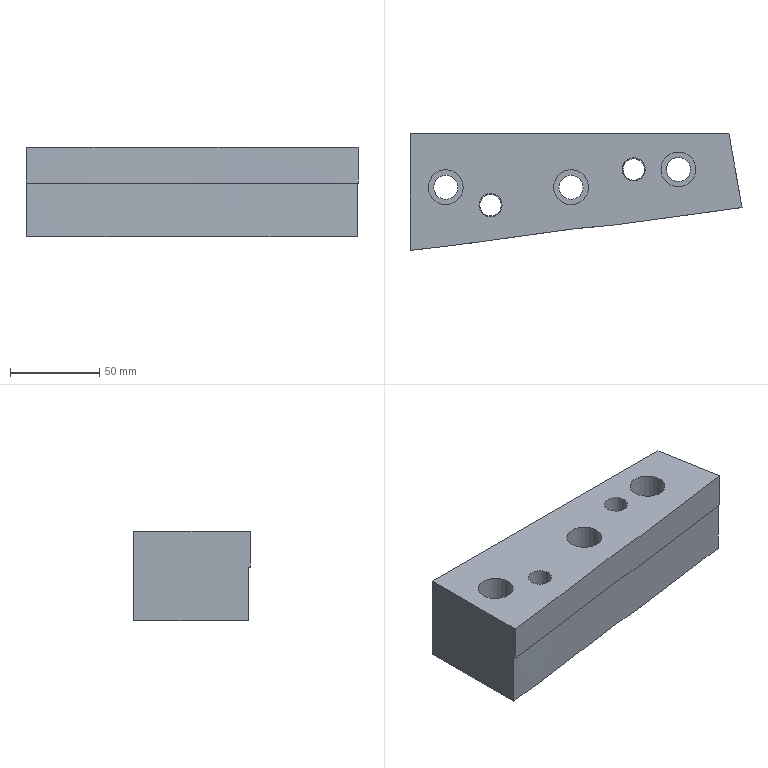Part | NX | features solid 2 | 1 solid | 23 faces | box 185.528 x 65.269 x 50 mm | volume 442182 mm3 | plane 11 | cylinder 10 | spline 2 | commonest cylinder face diameters 13.5 x3 19.5 x3 12 x2 13 x2
STEP:
#1=CARTESIAN_POINT('',(146.,-60.,-50.));
#2=VERTEX_POINT('',#1);
#3=CARTESIAN_POINT('',(140.,-60.,-50.));
#4=DIRECTION('',(0.,0.,1.));
#5=DIRECTION('',(1.,0.,0.));
#6=AXIS2_PLACEMENT_3D('',#3,#4,#5);
#7=CIRCLE('',#6,6.);
#8=EDGE_CURVE('',#2,#2,#7,.T.);
#9=ORIENTED_EDGE('',*,*,#8,.T.);
#10=EDGE_LOOP('',(#9));
#11=FACE_BOUND('',#10,.T.);
#12=CARTESIAN_POINT('',(226.,-40.,-50.));
#13=VERTEX_POINT('',#12);
#14=CARTESIAN_POINT('',(220.,-40.,-50.));
#15=DIRECTION('',(0.,0.,1.));
#16=DIRECTION('',(1.,0.,0.));
#17=AXIS2_PLACEMENT_3D('',#14,#15,#16);
#18=CIRCLE('',#17,6.);
#19=EDGE_CURVE('',#13,#13,#18,.T.);
#20=ORIENTED_EDGE('',*,*,#19,.T.);
#21=EDGE_LOOP('',(#20));
#22=FACE_BOUND('',#21,.T.);
#23=CARTESIAN_POINT('',(121.75,-50.,-50.));
#24=VERTEX_POINT('',#23);
#25=CARTESIAN_POINT('',(115.,-50.,-50.));
#26=DIRECTION('',(0.,0.,1.));
#27=DIRECTION('',(1.,0.,0.));
#28=AXIS2_PLACEMENT_3D('',#25,#26,#27);
#29=CIRCLE('',#28,6.75);
#30=EDGE_CURVE('',#24,#24,#29,.T.);
#31=ORIENTED_EDGE('',*,*,#30,.T.);
#32=EDGE_LOOP('',(#31));
#33=FACE_BOUND('',#32,.T.);
#34=CARTESIAN_POINT('',(191.75,-50.,-50.));
#35=VERTEX_POINT('',#34);
#36=CARTESIAN_POINT('',(185.,-50.,-50.));
#37=DIRECTION('',(0.,0.,1.));
#38=DIRECTION('',(1.,0.,0.));
#39=AXIS2_PLACEMENT_3D('',#36,#37,#38);
#40=CIRCLE('',#39,6.75);
#41=EDGE_CURVE('',#35,#35,#40,.T.);
#42=ORIENTED_EDGE('',*,*,#41,.T.);
#43=EDGE_LOOP('',(#42));
#44=FACE_BOUND('',#43,.T.);
#45=CARTESIAN_POINT('',(251.75,-40.,-50.));
#46=VERTEX_POINT('',#45);
#47=CARTESIAN_POINT('',(245.,-40.,-50.));
#48=DIRECTION('',(0.,0.,1.));
#49=DIRECTION('',(1.,0.,0.));
#50=AXIS2_PLACEMENT_3D('',#47,#48,#49);
#51=CIRCLE('',#50,6.75);
#52=EDGE_CURVE('',#46,#46,#51,.T.);
#53=ORIENTED_EDGE('',*,*,#52,.T.);
#54=EDGE_LOOP('',(#53));
#55=FACE_BOUND('',#54,.T.);
#56=CARTESIAN_POINT('',(280.354,-60.363,-50.));
#57=VERTEX_POINT('',#56);
#58=CARTESIAN_POINT('',(273.237,-20.,-50.));
#59=VERTEX_POINT('',#58);
#60=CARTESIAN_POINT('',(243.048,151.206,-50.));
#61=DIRECTION('',(-0.1736,0.9848,0.));
#62=VECTOR('',#61,1000.);
#63=LINE('',#60,#62);
#64=EDGE_CURVE('',#57,#59,#63,.T.);
#65=ORIENTED_EDGE('',*,*,#64,.F.);
#66=CARTESIAN_POINT('',(95.,-84.264,-50.));
#67=VERTEX_POINT('',#66);
#68=CARTESIAN_POINT('',(280.354,-60.363,-50.));
#69=CARTESIAN_POINT('',(272.636,-61.4,-50.));
#70=CARTESIAN_POINT('',(261.069,-63.03,-50.));
#71=CARTESIAN_POINT('',(245.641,-65.159,-50.));
#72=CARTESIAN_POINT('',(234.064,-66.718,-50.));
#73=CARTESIAN_POINT('',(222.493,-68.314,-50.));
#74=CARTESIAN_POINT('',(210.932,-69.992,-50.));
#75=CARTESIAN_POINT('',(199.277,-70.943,-50.));
#76=CARTESIAN_POINT('',(187.635,-71.985,-50.));
#77=CARTESIAN_POINT('',(176.074,-73.662,-50.));
#78=CARTESIAN_POINT('',(164.507,-75.298,-50.));
#79=CARTESIAN_POINT('',(152.929,-76.84,-50.));
#80=CARTESIAN_POINT('',(137.498,-78.952,-50.));
#81=CARTESIAN_POINT('',(118.23,-81.747,-50.));
#82=CARTESIAN_POINT('',(102.746,-83.443,-50.));
#83=CARTESIAN_POINT('',(95.,-84.264,-50.));
#84=B_SPLINE_CURVE_WITH_KNOTS('',3,(#68,#69,#70,#71,#72,#73,#74,#75,#76,#77,#78,#79,#80,#81,#82,#83),.UNSPECIFIED.,.F.,.F.,(4,1,1,1,1,1,1,1,1,1,1,1,1,4),(0.001298,0.02466,0.03634,0.04802,0.0597,0.07138,0.08306,0.09474,0.1064,0.1181,0.1298,0.1415,0.1648,0.1882),.UNSPECIFIED.);
#85=EDGE_CURVE('',#57,#67,#84,.T.);
#86=ORIENTED_EDGE('',*,*,#85,.T.);
#87=CARTESIAN_POINT('',(95.,-20.,-50.));
#88=VERTEX_POINT('',#87);
#89=CARTESIAN_POINT('',(95.,35.09,-50.));
#90=DIRECTION('',(0.,1.,0.));
#91=VECTOR('',#90,1000.);
#92=LINE('',#89,#91);
#93=EDGE_CURVE('',#67,#88,#92,.T.);
#94=ORIENTED_EDGE('',*,*,#93,.T.);
#95=CARTESIAN_POINT('',(-415.478,-20.,-50.));
#96=DIRECTION('',(-1.,0.,0.));
#97=VECTOR('',#96,1000.);
#98=LINE('',#95,#97);
#99=EDGE_CURVE('',#59,#88,#98,.T.);
#100=ORIENTED_EDGE('',*,*,#99,.F.);
#101=EDGE_LOOP('',(#65,#86,#94,#100));
#102=FACE_BOUND('',#101,.T.);
#103=CARTESIAN_POINT('',(-415.478,35.09,-50.));
#104=DIRECTION('',(0.,0.,1.));
#105=DIRECTION('',(1.,0.,0.));
#106=AXIS2_PLACEMENT_3D('',#103,#104,#105);
#107=PLANE('',#106);
#108=ADVANCED_FACE('',(#11,#22,#33,#44,#55,#102),#107,.F.);
#109=CARTESIAN_POINT('',(280.354,-60.363,-20.));
#110=VERTEX_POINT('',#109);
#111=CARTESIAN_POINT('',(280.528,-61.349,-20.));
#112=VERTEX_POINT('',#111);
#113=CARTESIAN_POINT('',(298.119,-161.113,-20.));
#114=DIRECTION('',(0.1736,-0.9848,0.));
#115=VECTOR('',#114,1000.);
#116=LINE('',#113,#115);
#117=EDGE_CURVE('',#110,#112,#116,.T.);
#118=ORIENTED_EDGE('',*,*,#117,.F.);
#119=CARTESIAN_POINT('',(280.354,-60.363,-60.));
#120=DIRECTION('',(0.,0.,-1.));
#121=VECTOR('',#120,1000.);
#122=LINE('',#119,#121);
#123=EDGE_CURVE('',#57,#110,#122,.F.);
#124=ORIENTED_EDGE('',*,*,#123,.F.);
#125=ORIENTED_EDGE('',*,*,#64,.T.);
#126=CARTESIAN_POINT('',(273.237,-20.,0.));
#127=VERTEX_POINT('',#126);
#128=CARTESIAN_POINT('',(273.237,-20.,0.));
#129=DIRECTION('',(0.,0.,-1.));
#130=VECTOR('',#129,1000.);
#131=LINE('',#128,#130);
#132=EDGE_CURVE('',#127,#59,#131,.T.);
#133=ORIENTED_EDGE('',*,*,#132,.F.);
#134=CARTESIAN_POINT('',(280.528,-61.349,0.));
#135=VERTEX_POINT('',#134);
#136=CARTESIAN_POINT('',(285.358,-88.743,0.));
#137=DIRECTION('',(0.1736,-0.9848,0.));
#138=VECTOR('',#137,1000.);
#139=LINE('',#136,#138);
#140=EDGE_CURVE('',#127,#135,#139,.T.);
#141=ORIENTED_EDGE('',*,*,#140,.T.);
#142=CARTESIAN_POINT('',(280.528,-61.349,-10.));
#143=DIRECTION('',(0.,0.,-1.));
#144=VECTOR('',#143,1000.);
#145=LINE('',#142,#144);
#146=EDGE_CURVE('',#135,#112,#145,.T.);
#147=ORIENTED_EDGE('',*,*,#146,.T.);
#148=EDGE_LOOP('',(#118,#124,#125,#133,#141,#147));
#149=FACE_BOUND('',#148,.T.);
#150=CARTESIAN_POINT('',(298.119,-161.113,0.));
#151=DIRECTION('',(0.9848,0.1736,0.));
#152=DIRECTION('',(-0.1736,0.9848,0.));
#153=AXIS2_PLACEMENT_3D('',#150,#151,#152);
#154=PLANE('',#153);
#155=ADVANCED_FACE('',(#149),#154,.T.);
#156=CARTESIAN_POINT('',(95.,-20.,0.));
#157=VERTEX_POINT('',#156);
#158=CARTESIAN_POINT('',(-470.381,-20.,0.));
#159=DIRECTION('',(1.,0.,0.));
#160=VECTOR('',#159,1000.);
#161=LINE('',#158,#160);
#162=EDGE_CURVE('',#157,#127,#161,.T.);
#163=ORIENTED_EDGE('',*,*,#162,.T.);
#164=ORIENTED_EDGE('',*,*,#132,.T.);
#165=ORIENTED_EDGE('',*,*,#99,.T.);
#166=CARTESIAN_POINT('',(95.,-20.,0.));
#167=DIRECTION('',(0.,0.,-1.));
#168=VECTOR('',#167,1000.);
#169=LINE('',#166,#168);
#170=EDGE_CURVE('',#157,#88,#169,.T.);
#171=ORIENTED_EDGE('',*,*,#170,.F.);
#172=EDGE_LOOP('',(#163,#164,#165,#171));
#173=FACE_BOUND('',#172,.T.);
#174=CARTESIAN_POINT('',(190.,-20.,0.));
#175=DIRECTION('',(0.,1.,0.));
#176=DIRECTION('',(0.,0.,1.));
#177=AXIS2_PLACEMENT_3D('',#174,#175,#176);
#178=PLANE('',#177);
#179=ADVANCED_FACE('',(#173),#178,.T.);
#180=CARTESIAN_POINT('',(95.,-85.269,0.));
#181=VERTEX_POINT('',#180);
#182=CARTESIAN_POINT('',(95.,-85.269,-20.));
#183=VERTEX_POINT('',#182);
#184=CARTESIAN_POINT('',(95.,-85.269,-10.));
#185=DIRECTION('',(0.,0.,-1.));
#186=VECTOR('',#185,1000.);
#187=LINE('',#184,#186);
#188=EDGE_CURVE('',#181,#183,#187,.T.);
#189=ORIENTED_EDGE('',*,*,#188,.T.);
#190=CARTESIAN_POINT('',(-190.231,-121.49,-20.));
#191=CARTESIAN_POINT('',(-188.654,-121.152,-20.));
#192=CARTESIAN_POINT('',(-185.47,-120.627,-20.));
#193=CARTESIAN_POINT('',(-180.656,-120.141,-20.));
#194=CARTESIAN_POINT('',(-175.882,-119.326,-20.));
#195=CARTESIAN_POINT('',(-169.679,-117.528,-20.));
#196=CARTESIAN_POINT('',(-162.185,-114.539,-20.));
#197=CARTESIAN_POINT('',(-153.086,-111.254,-20.));
#198=CARTESIAN_POINT('',(-144.031,-107.845,-20.));
#199=CARTESIAN_POINT('',(-136.465,-105.061,-20.));
#200=CARTESIAN_POINT('',(-130.418,-102.814,-20.));
#201=CARTESIAN_POINT('',(-125.812,-101.329,-20.));
#202=CARTESIAN_POINT('',(-121.306,-99.566,-20.));
#203=CARTESIAN_POINT('',(-116.876,-97.626,-20.));
#204=CARTESIAN_POINT('',(-112.335,-95.923,-20.));
#205=CARTESIAN_POINT('',(-107.564,-95.05,-20.));
#206=CARTESIAN_POINT('',(-102.756,-94.525,-20.));
#207=CARTESIAN_POINT('',(-96.349,-93.771,-20.));
#208=CARTESIAN_POINT('',(-89.902,-93.468,-20.));
#209=CARTESIAN_POINT('',(-83.452,-93.448,-20.));
#210=CARTESIAN_POINT('',(-77.002,-93.469,-20.));
#211=CARTESIAN_POINT('',(-68.939,-93.411,-20.));
#212=CARTESIAN_POINT('',(-56.04,-93.3,-20.));
#213=CARTESIAN_POINT('',(-33.465,-93.184,-20.));
#214=CARTESIAN_POINT('',(-7.666,-93.074,-20.));
#215=CARTESIAN_POINT('',(14.907,-92.653,-20.));
#216=CARTESIAN_POINT('',(27.794,-92.068,-20.));
#217=CARTESIAN_POINT('',(40.668,-91.245,-20.));
#218=CARTESIAN_POINT('',(51.917,-90.291,-20.));
#219=CARTESIAN_POINT('',(61.528,-89.174,-20.));
#220=CARTESIAN_POINT('',(67.939,-88.466,-20.));
#221=CARTESIAN_POINT('',(79.125,-86.95,-20.));
#222=CARTESIAN_POINT('',(95.161,-85.253,-20.));
#223=CARTESIAN_POINT('',(114.404,-83.21,-20.));
#224=CARTESIAN_POINT('',(133.568,-80.524,-20.));
#225=CARTESIAN_POINT('',(152.734,-77.861,-20.));
#226=CARTESIAN_POINT('',(171.916,-75.326,-20.));
#227=CARTESIAN_POINT('',(191.055,-72.413,-20.));
#228=CARTESIAN_POINT('',(207.17,-71.468,-20.));
#229=CARTESIAN_POINT('',(219.951,-69.697,-20.));
#230=CARTESIAN_POINT('',(232.724,-67.899,-20.));
#231=CARTESIAN_POINT('',(248.708,-65.766,-20.));
#232=CARTESIAN_POINT('',(267.87,-63.074,-20.));
#233=CARTESIAN_POINT('',(287.038,-60.44,-20.));
#234=CARTESIAN_POINT('',(301.448,-58.682,-20.));
#235=CARTESIAN_POINT('',(310.976,-56.987,-20.));
#236=CARTESIAN_POINT('',(314.916,-56.135,-20.));
#237=CARTESIAN_POINT('',(318.052,-55.382,-20.));
#238=CARTESIAN_POINT('',(320.39,-54.76,-20.));
#239=CARTESIAN_POINT('',(322.686,-53.981,-20.));
#240=CARTESIAN_POINT('',(325.595,-52.578,-20.));
#241=CARTESIAN_POINT('',(328.769,-50.098,-20.));
#242=CARTESIAN_POINT('',(332.247,-46.69,-20.));
#243=CARTESIAN_POINT('',(335.795,-43.406,-20.));
#244=CARTESIAN_POINT('',(343.661,-37.758,-20.));
#245=CARTESIAN_POINT('',(355.164,-28.914,-20.));
#246=CARTESIAN_POINT('',(370.422,-17.018,-20.));
#247=CARTESIAN_POINT('',(383.264,-7.249,-20.));
#248=CARTESIAN_POINT('',(392.416,-0.6713,-20.));
#249=CARTESIAN_POINT('',(396.953,2.733,-20.));
#250=CARTESIAN_POINT('',(398.886,5.372,-20.));
#251=CARTESIAN_POINT('',(399.725,7.654,-20.));
#252=CARTESIAN_POINT('',(399.76,10.078,-20.));
#253=CARTESIAN_POINT('',(399.483,13.317,-20.));
#254=CARTESIAN_POINT('',(399.712,17.34,-20.));
#255=CARTESIAN_POINT('',(399.612,22.179,-20.));
#256=CARTESIAN_POINT('',(399.633,31.854,-20.));
#257=CARTESIAN_POINT('',(399.593,46.366,-20.));
#258=CARTESIAN_POINT('',(399.637,62.491,-20.));
#259=CARTESIAN_POINT('',(399.588,73.779,-20.));
#260=CARTESIAN_POINT('',(399.652,79.422,-20.));
#261=CARTESIAN_POINT('',(399.59,82.647,-20.));
#262=CARTESIAN_POINT('',(399.564,85.065,-20.));
#263=CARTESIAN_POINT('',(399.725,87.486,-20.));
#264=CARTESIAN_POINT('',(399.756,89.902,-20.));
#265=CARTESIAN_POINT('',(399.247,92.301,-20.));
#266=CARTESIAN_POINT('',(397.362,95.008,-20.));
#267=CARTESIAN_POINT('',(393.635,96.774,-20.));
#268=CARTESIAN_POINT('',(389.279,98.826,-20.));
#269=CARTESIAN_POINT('',(384.732,100.498,-20.));
#270=CARTESIAN_POINT('',(378.765,102.95,-20.));
#271=CARTESIAN_POINT('',(362.589,110.229,-20.));
#272=CARTESIAN_POINT('',(344.928,118.135,-20.));
#273=CARTESIAN_POINT('',(327.281,126.072,-20.));
#274=CARTESIAN_POINT('',(319.932,129.381,-20.));
#275=CARTESIAN_POINT('',(314.075,132.102,-20.));
#276=CARTESIAN_POINT('',(309.387,133.376,-20.));
#277=CARTESIAN_POINT('',(304.547,133.785,-20.));
#278=CARTESIAN_POINT('',(299.716,133.401,-20.));
#279=CARTESIAN_POINT('',(294.929,132.704,-20.));
#280=CARTESIAN_POINT('',(288.543,131.8,-20.));
#281=CARTESIAN_POINT('',(277.364,130.241,-20.));
#282=CARTESIAN_POINT('',(242.2,125.552,-20.));
#283=CARTESIAN_POINT('',(184.637,118.048,-20.));
#284=CARTESIAN_POINT('',(120.701,109.541,-20.));
#285=CARTESIAN_POINT('',(69.531,102.902,-20.));
#286=CARTESIAN_POINT('',(40.777,98.94,-20.));
#287=CARTESIAN_POINT('',(21.566,96.615,-20.));
#288=CARTESIAN_POINT('',(8.743,95.212,-20.));
#289=CARTESIAN_POINT('',(-7.301,93.575,-20.));
#290=CARTESIAN_POINT('',(-26.625,92.505,-20.));
#291=CARTESIAN_POINT('',(-45.971,92.017,-20.));
#292=CARTESIAN_POINT('',(-62.09,91.675,-20.));
#293=CARTESIAN_POINT('',(-74.987,91.256,-20.));
#294=CARTESIAN_POINT('',(-84.664,91.165,-20.));
#295=CARTESIAN_POINT('',(-94.319,91.781,-20.));
#296=CARTESIAN_POINT('',(-103.929,92.966,-20.));
#297=CARTESIAN_POINT('',(-113.495,94.403,-20.));
#298=CARTESIAN_POINT('',(-119.856,95.492,-20.));
#299=CARTESIAN_POINT('',(-122.997,96.222,-20.));
#300=B_SPLINE_CURVE_WITH_KNOTS('',3,(#190,#191,#192,#193,#194,#195,#196,#197,#198,#199,#200,#201,#202,#203,#204,#205,#206,#207,#208,#209,#210,#211,#212,#213,#214,#215,#216,#217,#218,#219,#220,#221,#222,#223,#224,#225,#226,#227,#228,#229,#230,#231,#232,#233,#234,#235,#236,#237,#238,#239,#240,#241,#242,#243,#244,#245,#246,#247,#248,#249,#250,#251,#252,#253,#254,#255,#256,#257,#258,#259,#260,#261,#262,#263,#264,#265,#266,#267,#268,#269,#270,#271,#272,#273,#274,#275,#276,#277,#278,#279,#280,#281,#282,#283,#284,#285,#286,#287,#288,#289,#290,#291,#292,#293,#294,#295,#296,#297,#298,#299),.UNSPECIFIED.,.F.,.F.,(4,1,1,1,1,1,1,1,1,1,1,1,1,1,1,1,1,1,1,1,1,1,1,1,1,1,1,1,1,1,1,1,1,1,1,1,1,1,1,1,1,1,1,1,1,1,1,1,1,1,1,1,1,1,1,1,1,1,1,1,1,1,1,1,1,1,1,1,1,1,1,1,1,1,1,1,1,1,1,1,1,1,1,1,1,1,1,1,1,1,1,1,1,1,1,1,1,1,1,1,1,1,1,1,1,1,1,4),(0.4704,0.4724,0.4745,0.4766,0.4786,0.4828,0.4869,0.491,0.4952,0.4972,0.4993,0.5014,0.5035,0.5055,0.5076,0.5097,0.5117,0.5159,0.5179,0.52,0.5241,0.5283,0.5366,0.5531,0.5614,0.5655,0.5697,0.5779,0.58,0.5821,0.5862,0.5945,0.6028,0.611,0.6193,0.6276,0.6359,0.6441,0.6483,0.6524,0.6607,0.669,0.6772,0.6855,0.6876,0.6897,0.6907,0.6917,0.6928,0.6938,0.6959,0.6979,0.7,0.7021,0.7103,0.7186,0.7269,0.731,0.7331,0.7341,0.7352,0.7362,0.7372,0.7393,0.7414,0.7435,0.7517,0.76,0.7641,0.7662,0.7672,0.7683,0.7693,0.7703,0.7714,0.7724,0.7745,0.7766,0.7786,0.7807,0.7848,0.8014,0.8055,0.8097,0.8117,0.8138,0.8159,0.8179,0.82,0.8221,0.8262,0.8345,0.8676,0.9007,0.9172,0.9338,0.9379,0.9421,0.9503,0.9586,0.9669,0.9752,0.9793,0.9834,0.9876,0.9917,0.9959,1.),.UNSPECIFIED.);
#301=EDGE_CURVE('',#183,#112,#300,.T.);
#302=ORIENTED_EDGE('',*,*,#301,.T.);
#303=ORIENTED_EDGE('',*,*,#146,.F.);
#304=CARTESIAN_POINT('',(280.528,-61.349,0.));
#305=CARTESIAN_POINT('',(272.803,-62.386,0.));
#306=CARTESIAN_POINT('',(261.225,-64.018,0.));
#307=CARTESIAN_POINT('',(245.782,-66.149,0.));
#308=CARTESIAN_POINT('',(234.195,-67.709,0.));
#309=CARTESIAN_POINT('',(222.613,-69.308,0.));
#310=CARTESIAN_POINT('',(211.041,-70.986,0.));
#311=CARTESIAN_POINT('',(199.375,-71.938,0.));
#312=CARTESIAN_POINT('',(187.722,-72.982,0.));
#313=CARTESIAN_POINT('',(176.15,-74.662,0.));
#314=CARTESIAN_POINT('',(164.573,-76.298,0.));
#315=CARTESIAN_POINT('',(152.984,-77.842,0.));
#316=CARTESIAN_POINT('',(137.539,-79.956,0.));
#317=CARTESIAN_POINT('',(118.252,-82.754,0.));
#318=CARTESIAN_POINT('',(102.753,-84.448,0.));
#319=CARTESIAN_POINT('',(95.,-85.269,0.));
#320=B_SPLINE_CURVE_WITH_KNOTS('',3,(#304,#305,#306,#307,#308,#309,#310,#311,#312,#313,#314,#315,#316,#317,#318,#319),.UNSPECIFIED.,.F.,.F.,(4,1,1,1,1,1,1,1,1,1,1,1,1,4),(0.,0.02338,0.03507,0.04677,0.05846,0.07015,0.08184,0.09353,0.1052,0.1169,0.1286,0.1403,0.1637,0.1871),.UNSPECIFIED.);
#321=EDGE_CURVE('',#135,#181,#320,.T.);
#322=ORIENTED_EDGE('',*,*,#321,.T.);
#323=EDGE_LOOP('',(#189,#302,#303,#322));
#324=FACE_BOUND('',#323,.T.);
#325=CARTESIAN_POINT('',(95.,-85.269,0.));
#326=CARTESIAN_POINT('',(95.,-85.269,-20.));
#327=CARTESIAN_POINT('',(102.752,-84.448,0.));
#328=CARTESIAN_POINT('',(102.752,-84.448,-20.));
#329=CARTESIAN_POINT('',(118.251,-82.754,0.));
#330=CARTESIAN_POINT('',(118.251,-82.754,-20.));
#331=CARTESIAN_POINT('',(137.54,-79.956,0.));
#332=CARTESIAN_POINT('',(137.54,-79.956,-20.));
#333=CARTESIAN_POINT('',(152.986,-77.841,0.));
#334=CARTESIAN_POINT('',(152.986,-77.841,-20.));
#335=CARTESIAN_POINT('',(164.576,-76.298,0.));
#336=CARTESIAN_POINT('',(164.576,-76.298,-20.));
#337=CARTESIAN_POINT('',(176.156,-74.661,0.));
#338=CARTESIAN_POINT('',(176.156,-74.661,-20.));
#339=CARTESIAN_POINT('',(187.73,-72.981,0.));
#340=CARTESIAN_POINT('',(187.73,-72.981,-20.));
#341=CARTESIAN_POINT('',(199.376,-71.938,0.));
#342=CARTESIAN_POINT('',(199.376,-71.938,-20.));
#343=CARTESIAN_POINT('',(211.033,-70.987,0.));
#344=CARTESIAN_POINT('',(211.033,-70.987,-20.));
#345=CARTESIAN_POINT('',(222.609,-69.308,0.));
#346=CARTESIAN_POINT('',(222.609,-69.308,-20.));
#347=CARTESIAN_POINT('',(234.191,-67.71,0.));
#348=CARTESIAN_POINT('',(234.191,-67.71,-20.));
#349=CARTESIAN_POINT('',(245.779,-66.15,0.));
#350=CARTESIAN_POINT('',(245.779,-66.15,-20.));
#351=CARTESIAN_POINT('',(261.224,-64.018,0.));
#352=CARTESIAN_POINT('',(261.224,-64.018,-20.));
#353=CARTESIAN_POINT('',(272.802,-62.386,0.));
#354=CARTESIAN_POINT('',(272.802,-62.386,-20.));
#355=CARTESIAN_POINT('',(280.528,-61.349,0.));
#356=CARTESIAN_POINT('',(280.528,-61.349,-20.));
#357=B_SPLINE_SURFACE_WITH_KNOTS('',3,1,((#325,#326),(#327,#328),(#329,#330),(#331,#332),(#333,#334),(#335,#336),(#337,#338),(#339,#340),(#341,#342),(#343,#344),(#345,#346),(#347,#348),(#349,#350),(#351,#352),(#353,#354),(#355,#356)),.SURF_OF_LINEAR_EXTRUSION.,.F.,.F.,.F.,(4,1,1,1,1,1,1,1,1,1,1,1,1,4),(2,2),(0.5944,0.6044,0.6144,0.6194,0.6244,0.6294,0.6344,0.6394,0.6444,0.6494,0.6544,0.6594,0.6644,0.6744),(0.,1.),.UNSPECIFIED.);
#358=ADVANCED_FACE('',(#324),#357,.F.);
#359=CARTESIAN_POINT('',(133.5,-60.,0.));
#360=VERTEX_POINT('',#359);
#361=CARTESIAN_POINT('',(140.,-60.,0.));
#362=DIRECTION('',(0.,0.,-1.));
#363=DIRECTION('',(-1.,0.,0.));
#364=AXIS2_PLACEMENT_3D('',#361,#362,#363);
#365=CIRCLE('',#364,6.5);
#366=EDGE_CURVE('',#360,#360,#365,.T.);
#367=ORIENTED_EDGE('',*,*,#366,.T.);
#368=EDGE_LOOP('',(#367));
#369=FACE_BOUND('',#368,.T.);
#370=CARTESIAN_POINT('',(213.5,-40.,0.));
#371=VERTEX_POINT('',#370);
#372=CARTESIAN_POINT('',(220.,-40.,0.));
#373=DIRECTION('',(0.,0.,-1.));
#374=DIRECTION('',(-1.,0.,0.));
#375=AXIS2_PLACEMENT_3D('',#372,#373,#374);
#376=CIRCLE('',#375,6.5);
#377=EDGE_CURVE('',#371,#371,#376,.T.);
#378=ORIENTED_EDGE('',*,*,#377,.T.);
#379=EDGE_LOOP('',(#378));
#380=FACE_BOUND('',#379,.T.);
#381=CARTESIAN_POINT('',(105.25,-50.,0.));
#382=VERTEX_POINT('',#381);
#383=CARTESIAN_POINT('',(115.,-50.,0.));
#384=DIRECTION('',(0.,0.,-1.));
#385=DIRECTION('',(-1.,0.,0.));
#386=AXIS2_PLACEMENT_3D('',#383,#384,#385);
#387=CIRCLE('',#386,9.75);
#388=EDGE_CURVE('',#382,#382,#387,.T.);
#389=ORIENTED_EDGE('',*,*,#388,.T.);
#390=EDGE_LOOP('',(#389));
#391=FACE_BOUND('',#390,.T.);
#392=CARTESIAN_POINT('',(175.25,-50.,0.));
#393=VERTEX_POINT('',#392);
#394=CARTESIAN_POINT('',(185.,-50.,0.));
#395=DIRECTION('',(0.,0.,-1.));
#396=DIRECTION('',(-1.,0.,0.));
#397=AXIS2_PLACEMENT_3D('',#394,#395,#396);
#398=CIRCLE('',#397,9.75);
#399=EDGE_CURVE('',#393,#393,#398,.T.);
#400=ORIENTED_EDGE('',*,*,#399,.T.);
#401=EDGE_LOOP('',(#400));
#402=FACE_BOUND('',#401,.T.);
#403=CARTESIAN_POINT('',(235.25,-40.,0.));
#404=VERTEX_POINT('',#403);
#405=CARTESIAN_POINT('',(245.,-40.,0.));
#406=DIRECTION('',(0.,0.,-1.));
#407=DIRECTION('',(-1.,0.,0.));
#408=AXIS2_PLACEMENT_3D('',#405,#406,#407);
#409=CIRCLE('',#408,9.75);
#410=EDGE_CURVE('',#404,#404,#409,.T.);
#411=ORIENTED_EDGE('',*,*,#410,.T.);
#412=EDGE_LOOP('',(#411));
#413=FACE_BOUND('',#412,.T.);
#414=ORIENTED_EDGE('',*,*,#140,.F.);
#415=ORIENTED_EDGE('',*,*,#162,.F.);
#416=CARTESIAN_POINT('',(95.,-222.,0.));
#417=DIRECTION('',(0.,-1.,0.));
#418=VECTOR('',#417,1000.);
#419=LINE('',#416,#418);
#420=EDGE_CURVE('',#157,#181,#419,.T.);
#421=ORIENTED_EDGE('',*,*,#420,.T.);
#422=ORIENTED_EDGE('',*,*,#321,.F.);
#423=EDGE_LOOP('',(#414,#415,#421,#422));
#424=FACE_BOUND('',#423,.T.);
#425=CARTESIAN_POINT('',(-470.381,-222.,0.));
#426=DIRECTION('',(0.,0.,-1.));
#427=DIRECTION('',(-1.,0.,0.));
#428=AXIS2_PLACEMENT_3D('',#425,#426,#427);
#429=PLANE('',#428);
#430=ADVANCED_FACE('',(#369,#380,#391,#402,#413,#424),#429,.F.);
#431=CARTESIAN_POINT('',(95.,-84.264,-20.));
#432=VERTEX_POINT('',#431);
#433=CARTESIAN_POINT('',(95.,-84.264,-60.));
#434=DIRECTION('',(0.,0.,-1.));
#435=VECTOR('',#434,1000.);
#436=LINE('',#433,#435);
#437=EDGE_CURVE('',#67,#432,#436,.F.);
#438=ORIENTED_EDGE('',*,*,#437,.T.);
#439=CARTESIAN_POINT('',(95.,83.097,-20.));
#440=DIRECTION('',(0.,-1.,0.));
#441=VECTOR('',#440,1000.);
#442=LINE('',#439,#441);
#443=EDGE_CURVE('',#432,#183,#442,.T.);
#444=ORIENTED_EDGE('',*,*,#443,.T.);
#445=ORIENTED_EDGE('',*,*,#188,.F.);
#446=ORIENTED_EDGE('',*,*,#420,.F.);
#447=ORIENTED_EDGE('',*,*,#170,.T.);
#448=ORIENTED_EDGE('',*,*,#93,.F.);
#449=EDGE_LOOP('',(#438,#444,#445,#446,#447,#448));
#450=FACE_BOUND('',#449,.T.);
#451=CARTESIAN_POINT('',(95.,83.097,-25.));
#452=DIRECTION('',(1.,0.,0.));
#453=DIRECTION('',(0.,0.,-1.));
#454=AXIS2_PLACEMENT_3D('',#451,#452,#453);
#455=PLANE('',#454);
#456=ADVANCED_FACE('',(#450),#455,.F.);
#457=CARTESIAN_POINT('',(238.25,-40.,-15.));
#458=VERTEX_POINT('',#457);
#459=CARTESIAN_POINT('',(245.,-40.,-15.));
#460=DIRECTION('',(0.,0.,-1.));
#461=DIRECTION('',(-1.,0.,0.));
#462=AXIS2_PLACEMENT_3D('',#459,#460,#461);
#463=CIRCLE('',#462,6.75);
#464=EDGE_CURVE('',#458,#458,#463,.T.);
#465=ORIENTED_EDGE('',*,*,#464,.F.);
#466=EDGE_LOOP('',(#465));
#467=FACE_BOUND('',#466,.T.);
#468=ORIENTED_EDGE('',*,*,#52,.F.);
#469=EDGE_LOOP('',(#468));
#470=FACE_BOUND('',#469,.T.);
#471=CARTESIAN_POINT('',(245.,-40.,-100.));
#472=DIRECTION('',(0.,0.,-1.));
#473=DIRECTION('',(-1.,0.,0.));
#474=AXIS2_PLACEMENT_3D('',#471,#472,#473);
#475=CYLINDRICAL_SURFACE('',#474,6.75);
#476=ADVANCED_FACE('',(#467,#470),#475,.F.);
#477=ORIENTED_EDGE('',*,*,#464,.T.);
#478=EDGE_LOOP('',(#477));
#479=FACE_BOUND('',#478,.T.);
#480=CARTESIAN_POINT('',(235.25,-40.,-15.));
#481=VERTEX_POINT('',#480);
#482=CARTESIAN_POINT('',(245.,-40.,-15.));
#483=DIRECTION('',(0.,0.,-1.));
#484=DIRECTION('',(-1.,0.,0.));
#485=AXIS2_PLACEMENT_3D('',#482,#483,#484);
#486=CIRCLE('',#485,9.75);
#487=EDGE_CURVE('',#481,#481,#486,.T.);
#488=ORIENTED_EDGE('',*,*,#487,.F.);
#489=EDGE_LOOP('',(#488));
#490=FACE_BOUND('',#489,.T.);
#491=CARTESIAN_POINT('',(245.,-40.,-15.));
#492=DIRECTION('',(0.,0.,-1.));
#493=DIRECTION('',(-1.,0.,0.));
#494=AXIS2_PLACEMENT_3D('',#491,#492,#493);
#495=PLANE('',#494);
#496=ADVANCED_FACE('',(#479,#490),#495,.F.);
#497=ORIENTED_EDGE('',*,*,#487,.T.);
#498=EDGE_LOOP('',(#497));
#499=FACE_BOUND('',#498,.T.);
#500=ORIENTED_EDGE('',*,*,#410,.F.);
#501=EDGE_LOOP('',(#500));
#502=FACE_BOUND('',#501,.T.);
#503=CARTESIAN_POINT('',(245.,-40.,0.));
#504=DIRECTION('',(0.,0.,-1.));
#505=DIRECTION('',(-1.,0.,0.));
#506=AXIS2_PLACEMENT_3D('',#503,#504,#505);
#507=CYLINDRICAL_SURFACE('',#506,9.75);
#508=ADVANCED_FACE('',(#499,#502),#507,.F.);
#509=CARTESIAN_POINT('',(178.25,-50.,-15.));
#510=VERTEX_POINT('',#509);
#511=CARTESIAN_POINT('',(185.,-50.,-15.));
#512=DIRECTION('',(0.,0.,-1.));
#513=DIRECTION('',(-1.,0.,0.));
#514=AXIS2_PLACEMENT_3D('',#511,#512,#513);
#515=CIRCLE('',#514,6.75);
#516=EDGE_CURVE('',#510,#510,#515,.T.);
#517=ORIENTED_EDGE('',*,*,#516,.F.);
#518=EDGE_LOOP('',(#517));
#519=FACE_BOUND('',#518,.T.);
#520=ORIENTED_EDGE('',*,*,#41,.F.);
#521=EDGE_LOOP('',(#520));
#522=FACE_BOUND('',#521,.T.);
#523=CARTESIAN_POINT('',(185.,-50.,-100.));
#524=DIRECTION('',(0.,0.,-1.));
#525=DIRECTION('',(-1.,0.,0.));
#526=AXIS2_PLACEMENT_3D('',#523,#524,#525);
#527=CYLINDRICAL_SURFACE('',#526,6.75);
#528=ADVANCED_FACE('',(#519,#522),#527,.F.);
#529=ORIENTED_EDGE('',*,*,#516,.T.);
#530=EDGE_LOOP('',(#529));
#531=FACE_BOUND('',#530,.T.);
#532=CARTESIAN_POINT('',(175.25,-50.,-15.));
#533=VERTEX_POINT('',#532);
#534=CARTESIAN_POINT('',(185.,-50.,-15.));
#535=DIRECTION('',(0.,0.,-1.));
#536=DIRECTION('',(-1.,0.,0.));
#537=AXIS2_PLACEMENT_3D('',#534,#535,#536);
#538=CIRCLE('',#537,9.75);
#539=EDGE_CURVE('',#533,#533,#538,.T.);
#540=ORIENTED_EDGE('',*,*,#539,.F.);
#541=EDGE_LOOP('',(#540));
#542=FACE_BOUND('',#541,.T.);
#543=CARTESIAN_POINT('',(185.,-60.,-15.));
#544=DIRECTION('',(0.,0.,-1.));
#545=DIRECTION('',(-1.,0.,0.));
#546=AXIS2_PLACEMENT_3D('',#543,#544,#545);
#547=PLANE('',#546);
#548=ADVANCED_FACE('',(#531,#542),#547,.F.);
#549=ORIENTED_EDGE('',*,*,#539,.T.);
#550=EDGE_LOOP('',(#549));
#551=FACE_BOUND('',#550,.T.);
#552=ORIENTED_EDGE('',*,*,#399,.F.);
#553=EDGE_LOOP('',(#552));
#554=FACE_BOUND('',#553,.T.);
#555=CARTESIAN_POINT('',(185.,-50.,0.));
#556=DIRECTION('',(0.,0.,-1.));
#557=DIRECTION('',(-1.,0.,0.));
#558=AXIS2_PLACEMENT_3D('',#555,#556,#557);
#559=CYLINDRICAL_SURFACE('',#558,9.75);
#560=ADVANCED_FACE('',(#551,#554),#559,.F.);
#561=CARTESIAN_POINT('',(108.25,-50.,-15.));
#562=VERTEX_POINT('',#561);
#563=CARTESIAN_POINT('',(115.,-50.,-15.));
#564=DIRECTION('',(0.,0.,-1.));
#565=DIRECTION('',(-1.,0.,0.));
#566=AXIS2_PLACEMENT_3D('',#563,#564,#565);
#567=CIRCLE('',#566,6.75);
#568=EDGE_CURVE('',#562,#562,#567,.T.);
#569=ORIENTED_EDGE('',*,*,#568,.F.);
#570=EDGE_LOOP('',(#569));
#571=FACE_BOUND('',#570,.T.);
#572=ORIENTED_EDGE('',*,*,#30,.F.);
#573=EDGE_LOOP('',(#572));
#574=FACE_BOUND('',#573,.T.);
#575=CARTESIAN_POINT('',(115.,-50.,-100.));
#576=DIRECTION('',(0.,0.,-1.));
#577=DIRECTION('',(-1.,0.,0.));
#578=AXIS2_PLACEMENT_3D('',#575,#576,#577);
#579=CYLINDRICAL_SURFACE('',#578,6.75);
#580=ADVANCED_FACE('',(#571,#574),#579,.F.);
#581=ORIENTED_EDGE('',*,*,#568,.T.);
#582=EDGE_LOOP('',(#581));
#583=FACE_BOUND('',#582,.T.);
#584=CARTESIAN_POINT('',(105.25,-50.,-15.));
#585=VERTEX_POINT('',#584);
#586=CARTESIAN_POINT('',(115.,-50.,-15.));
#587=DIRECTION('',(0.,0.,-1.));
#588=DIRECTION('',(-1.,0.,0.));
#589=AXIS2_PLACEMENT_3D('',#586,#587,#588);
#590=CIRCLE('',#589,9.75);
#591=EDGE_CURVE('',#585,#585,#590,.T.);
#592=ORIENTED_EDGE('',*,*,#591,.F.);
#593=EDGE_LOOP('',(#592));
#594=FACE_BOUND('',#593,.T.);
#595=CARTESIAN_POINT('',(115.,-50.,-15.));
#596=DIRECTION('',(0.,0.,-1.));
#597=DIRECTION('',(-1.,0.,0.));
#598=AXIS2_PLACEMENT_3D('',#595,#596,#597);
#599=PLANE('',#598);
#600=ADVANCED_FACE('',(#583,#594),#599,.F.);
#601=ORIENTED_EDGE('',*,*,#591,.T.);
#602=EDGE_LOOP('',(#601));
#603=FACE_BOUND('',#602,.T.);
#604=ORIENTED_EDGE('',*,*,#388,.F.);
#605=EDGE_LOOP('',(#604));
#606=FACE_BOUND('',#605,.T.);
#607=CARTESIAN_POINT('',(115.,-50.,0.));
#608=DIRECTION('',(0.,0.,-1.));
#609=DIRECTION('',(-1.,0.,0.));
#610=AXIS2_PLACEMENT_3D('',#607,#608,#609);
#611=CYLINDRICAL_SURFACE('',#610,9.75);
#612=ADVANCED_FACE('',(#603,#606),#611,.F.);
#613=CARTESIAN_POINT('',(214.,-40.,-20.));
#614=VERTEX_POINT('',#613);
#615=CARTESIAN_POINT('',(220.,-40.,-20.));
#616=DIRECTION('',(0.,0.,-1.));
#617=DIRECTION('',(-1.,0.,0.));
#618=AXIS2_PLACEMENT_3D('',#615,#616,#617);
#619=CIRCLE('',#618,6.);
#620=EDGE_CURVE('',#614,#614,#619,.T.);
#621=ORIENTED_EDGE('',*,*,#620,.F.);
#622=EDGE_LOOP('',(#621));
#623=FACE_BOUND('',#622,.T.);
#624=ORIENTED_EDGE('',*,*,#19,.F.);
#625=EDGE_LOOP('',(#624));
#626=FACE_BOUND('',#625,.T.);
#627=CARTESIAN_POINT('',(220.,-40.,-100.));
#628=DIRECTION('',(0.,0.,-1.));
#629=DIRECTION('',(-1.,0.,0.));
#630=AXIS2_PLACEMENT_3D('',#627,#628,#629);
#631=CYLINDRICAL_SURFACE('',#630,6.);
#632=ADVANCED_FACE('',(#623,#626),#631,.F.);
#633=ORIENTED_EDGE('',*,*,#620,.T.);
#634=EDGE_LOOP('',(#633));
#635=FACE_BOUND('',#634,.T.);
#636=CARTESIAN_POINT('',(213.5,-40.,-20.));
#637=VERTEX_POINT('',#636);
#638=CARTESIAN_POINT('',(220.,-40.,-20.));
#639=DIRECTION('',(0.,0.,-1.));
#640=DIRECTION('',(-1.,0.,0.));
#641=AXIS2_PLACEMENT_3D('',#638,#639,#640);
#642=CIRCLE('',#641,6.5);
#643=EDGE_CURVE('',#637,#637,#642,.T.);
#644=ORIENTED_EDGE('',*,*,#643,.F.);
#645=EDGE_LOOP('',(#644));
#646=FACE_BOUND('',#645,.T.);
#647=CARTESIAN_POINT('',(220.,-40.,-20.));
#648=DIRECTION('',(0.,0.,-1.));
#649=DIRECTION('',(-1.,0.,0.));
#650=AXIS2_PLACEMENT_3D('',#647,#648,#649);
#651=PLANE('',#650);
#652=ADVANCED_FACE('',(#635,#646),#651,.F.);
#653=ORIENTED_EDGE('',*,*,#643,.T.);
#654=EDGE_LOOP('',(#653));
#655=FACE_BOUND('',#654,.T.);
#656=ORIENTED_EDGE('',*,*,#377,.F.);
#657=EDGE_LOOP('',(#656));
#658=FACE_BOUND('',#657,.T.);
#659=CARTESIAN_POINT('',(220.,-40.,0.));
#660=DIRECTION('',(0.,0.,-1.));
#661=DIRECTION('',(-1.,0.,0.));
#662=AXIS2_PLACEMENT_3D('',#659,#660,#661);
#663=CYLINDRICAL_SURFACE('',#662,6.5);
#664=ADVANCED_FACE('',(#655,#658),#663,.F.);
#665=CARTESIAN_POINT('',(134.,-60.,-20.));
#666=VERTEX_POINT('',#665);
#667=CARTESIAN_POINT('',(140.,-60.,-20.));
#668=DIRECTION('',(0.,0.,-1.));
#669=DIRECTION('',(-1.,0.,0.));
#670=AXIS2_PLACEMENT_3D('',#667,#668,#669);
#671=CIRCLE('',#670,6.);
#672=EDGE_CURVE('',#666,#666,#671,.T.);
#673=ORIENTED_EDGE('',*,*,#672,.F.);
#674=EDGE_LOOP('',(#673));
#675=FACE_BOUND('',#674,.T.);
#676=ORIENTED_EDGE('',*,*,#8,.F.);
#677=EDGE_LOOP('',(#676));
#678=FACE_BOUND('',#677,.T.);
#679=CARTESIAN_POINT('',(140.,-60.,-100.));
#680=DIRECTION('',(0.,0.,-1.));
#681=DIRECTION('',(-1.,0.,0.));
#682=AXIS2_PLACEMENT_3D('',#679,#680,#681);
#683=CYLINDRICAL_SURFACE('',#682,6.);
#684=ADVANCED_FACE('',(#675,#678),#683,.F.);
#685=ORIENTED_EDGE('',*,*,#672,.T.);
#686=EDGE_LOOP('',(#685));
#687=FACE_BOUND('',#686,.T.);
#688=CARTESIAN_POINT('',(133.5,-60.,-20.));
#689=VERTEX_POINT('',#688);
#690=CARTESIAN_POINT('',(140.,-60.,-20.));
#691=DIRECTION('',(0.,0.,-1.));
#692=DIRECTION('',(-1.,0.,0.));
#693=AXIS2_PLACEMENT_3D('',#690,#691,#692);
#694=CIRCLE('',#693,6.5);
#695=EDGE_CURVE('',#689,#689,#694,.T.);
#696=ORIENTED_EDGE('',*,*,#695,.F.);
#697=EDGE_LOOP('',(#696));
#698=FACE_BOUND('',#697,.T.);
#699=CARTESIAN_POINT('',(140.,-60.,-20.));
#700=DIRECTION('',(0.,0.,-1.));
#701=DIRECTION('',(-1.,0.,0.));
#702=AXIS2_PLACEMENT_3D('',#699,#700,#701);
#703=PLANE('',#702);
#704=ADVANCED_FACE('',(#687,#698),#703,.F.);
#705=ORIENTED_EDGE('',*,*,#695,.T.);
#706=EDGE_LOOP('',(#705));
#707=FACE_BOUND('',#706,.T.);
#708=ORIENTED_EDGE('',*,*,#366,.F.);
#709=EDGE_LOOP('',(#708));
#710=FACE_BOUND('',#709,.T.);
#711=CARTESIAN_POINT('',(140.,-60.,0.));
#712=DIRECTION('',(0.,0.,-1.));
#713=DIRECTION('',(-1.,0.,0.));
#714=AXIS2_PLACEMENT_3D('',#711,#712,#713);
#715=CYLINDRICAL_SURFACE('',#714,6.5);
#716=ADVANCED_FACE('',(#707,#710),#715,.F.);
#717=ORIENTED_EDGE('',*,*,#123,.T.);
#718=CARTESIAN_POINT('',(95.,-84.264,-20.));
#719=CARTESIAN_POINT('',(102.746,-83.443,-20.));
#720=CARTESIAN_POINT('',(118.203,-81.751,-20.));
#721=CARTESIAN_POINT('',(137.472,-78.956,-20.));
#722=CARTESIAN_POINT('',(152.912,-76.842,-20.));
#723=CARTESIAN_POINT('',(164.495,-75.3,-20.));
#724=CARTESIAN_POINT('',(176.048,-73.666,-20.));
#725=CARTESIAN_POINT('',(187.637,-71.984,-20.));
#726=CARTESIAN_POINT('',(199.335,-70.938,-20.));
#727=CARTESIAN_POINT('',(210.927,-69.992,-20.));
#728=CARTESIAN_POINT('',(222.469,-68.318,-20.));
#729=CARTESIAN_POINT('',(234.053,-66.719,-20.));
#730=CARTESIAN_POINT('',(245.632,-65.161,-20.));
#731=CARTESIAN_POINT('',(261.058,-63.032,-20.));
#732=CARTESIAN_POINT('',(272.63,-61.401,-20.));
#733=CARTESIAN_POINT('',(280.354,-60.363,-20.));
#734=B_SPLINE_CURVE_WITH_KNOTS('',3,(#718,#719,#720,#721,#722,#723,#724,#725,#726,#727,#728,#729,#730,#731,#732,#733),.UNSPECIFIED.,.F.,.F.,(4,1,1,1,1,1,1,1,1,1,1,1,1,4),(0.5945,0.6045,0.6145,0.6194,0.6244,0.6294,0.6344,0.6394,0.6444,0.6494,0.6544,0.6594,0.6644,0.6744),.UNSPECIFIED.);
#735=EDGE_CURVE('',#432,#110,#734,.T.);
#736=ORIENTED_EDGE('',*,*,#735,.F.);
#737=ORIENTED_EDGE('',*,*,#437,.F.);
#738=ORIENTED_EDGE('',*,*,#85,.F.);
#739=EDGE_LOOP('',(#717,#736,#737,#738));
#740=FACE_BOUND('',#739,.T.);
#741=CARTESIAN_POINT('',(95.,-84.264,-20.));
#742=CARTESIAN_POINT('',(95.,-84.264,-50.));
#743=CARTESIAN_POINT('',(102.746,-83.443,-20.));
#744=CARTESIAN_POINT('',(102.746,-83.443,-50.));
#745=CARTESIAN_POINT('',(118.203,-81.751,-20.));
#746=CARTESIAN_POINT('',(118.203,-81.751,-50.));
#747=CARTESIAN_POINT('',(137.472,-78.956,-20.));
#748=CARTESIAN_POINT('',(137.472,-78.956,-50.));
#749=CARTESIAN_POINT('',(152.912,-76.842,-20.));
#750=CARTESIAN_POINT('',(152.912,-76.842,-50.));
#751=CARTESIAN_POINT('',(164.495,-75.3,-20.));
#752=CARTESIAN_POINT('',(164.495,-75.3,-50.));
#753=CARTESIAN_POINT('',(176.048,-73.666,-20.));
#754=CARTESIAN_POINT('',(176.048,-73.666,-50.));
#755=CARTESIAN_POINT('',(187.637,-71.984,-20.));
#756=CARTESIAN_POINT('',(187.637,-71.984,-50.));
#757=CARTESIAN_POINT('',(199.335,-70.938,-20.));
#758=CARTESIAN_POINT('',(199.335,-70.938,-50.));
#759=CARTESIAN_POINT('',(210.927,-69.992,-20.));
#760=CARTESIAN_POINT('',(210.927,-69.992,-50.));
#761=CARTESIAN_POINT('',(222.469,-68.318,-20.));
#762=CARTESIAN_POINT('',(222.469,-68.318,-50.));
#763=CARTESIAN_POINT('',(234.053,-66.719,-20.));
#764=CARTESIAN_POINT('',(234.053,-66.719,-50.));
#765=CARTESIAN_POINT('',(245.632,-65.161,-20.));
#766=CARTESIAN_POINT('',(245.632,-65.161,-50.));
#767=CARTESIAN_POINT('',(261.058,-63.032,-20.));
#768=CARTESIAN_POINT('',(261.058,-63.032,-50.));
#769=CARTESIAN_POINT('',(272.63,-61.401,-20.));
#770=CARTESIAN_POINT('',(272.63,-61.401,-50.));
#771=CARTESIAN_POINT('',(280.354,-60.363,-20.));
#772=CARTESIAN_POINT('',(280.354,-60.363,-50.));
#773=B_SPLINE_SURFACE_WITH_KNOTS('',3,1,((#741,#742),(#743,#744),(#745,#746),(#747,#748),(#749,#750),(#751,#752),(#753,#754),(#755,#756),(#757,#758),(#759,#760),(#761,#762),(#763,#764),(#765,#766),(#767,#768),(#769,#770),(#771,#772)),.SURF_OF_LINEAR_EXTRUSION.,.F.,.F.,.F.,(4,1,1,1,1,1,1,1,1,1,1,1,1,4),(2,2),(0.5945,0.6045,0.6145,0.6194,0.6244,0.6294,0.6344,0.6394,0.6444,0.6494,0.6544,0.6594,0.6644,0.6744),(0.,1.),.UNSPECIFIED.);
#774=ADVANCED_FACE('',(#740),#773,.F.);
#775=ORIENTED_EDGE('',*,*,#117,.T.);
#776=ORIENTED_EDGE('',*,*,#301,.F.);
#777=ORIENTED_EDGE('',*,*,#443,.F.);
#778=ORIENTED_EDGE('',*,*,#735,.T.);
#779=EDGE_LOOP('',(#775,#776,#777,#778));
#780=FACE_BOUND('',#779,.T.);
#781=CARTESIAN_POINT('',(-190.231,-121.49,-20.));
#782=DIRECTION('',(0.,0.,1.));
#783=DIRECTION('',(1.,0.,0.));
#784=AXIS2_PLACEMENT_3D('',#781,#782,#783);
#785=PLANE('',#784);
#786=ADVANCED_FACE('',(#780),#785,.F.);
#787=CLOSED_SHELL('',(#108,#155,#179,#358,#430,#456,#476,#496,#508,#528,#548,#560,#580,#600,#612,#632,#652,#664,#684,#704,#716,#774,#786));
#788=MANIFOLD_SOLID_BREP('',#787);
#789=(LENGTH_UNIT()NAMED_UNIT(*)SI_UNIT(.MILLI.,.METRE.));
#790=UNCERTAINTY_MEASURE_WITH_UNIT(LENGTH_MEASURE(0.0508),#789,'','');
#791=(NAMED_UNIT(*)PLANE_ANGLE_UNIT()SI_UNIT($,.RADIAN.));
#792=(NAMED_UNIT(*)SI_UNIT($,.STERADIAN.)SOLID_ANGLE_UNIT());
#793=(GEOMETRIC_REPRESENTATION_CONTEXT(3)GLOBAL_UNCERTAINTY_ASSIGNED_CONTEXT((#790))GLOBAL_UNIT_ASSIGNED_CONTEXT((#789,#791,#792))REPRESENTATION_CONTEXT('',''));
#794=ADVANCED_BREP_SHAPE_REPRESENTATION('',(#788),#793);